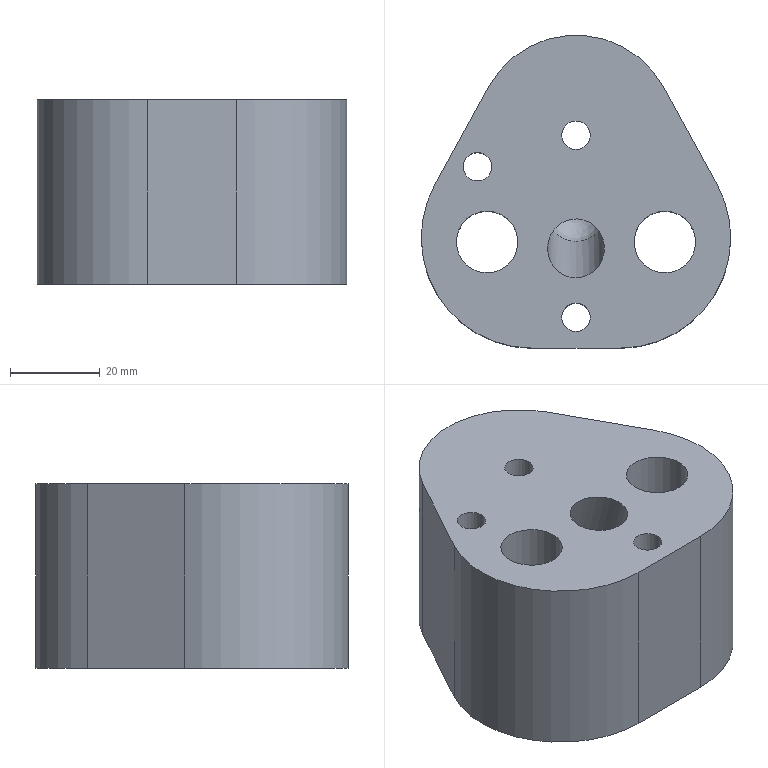Part | STEP file | 1_id658_x_t | 1 solid | 21 faces | box 69.088 x 69.85 x 41.275 mm | volume 100264 mm3 | cylinder 12 | plane 8 | sphere 1 | commonest cylinder face diameters 6.35 x3 13.741 x2 20.218 x2 49.276 x2 12.7 x1 31.75 x1